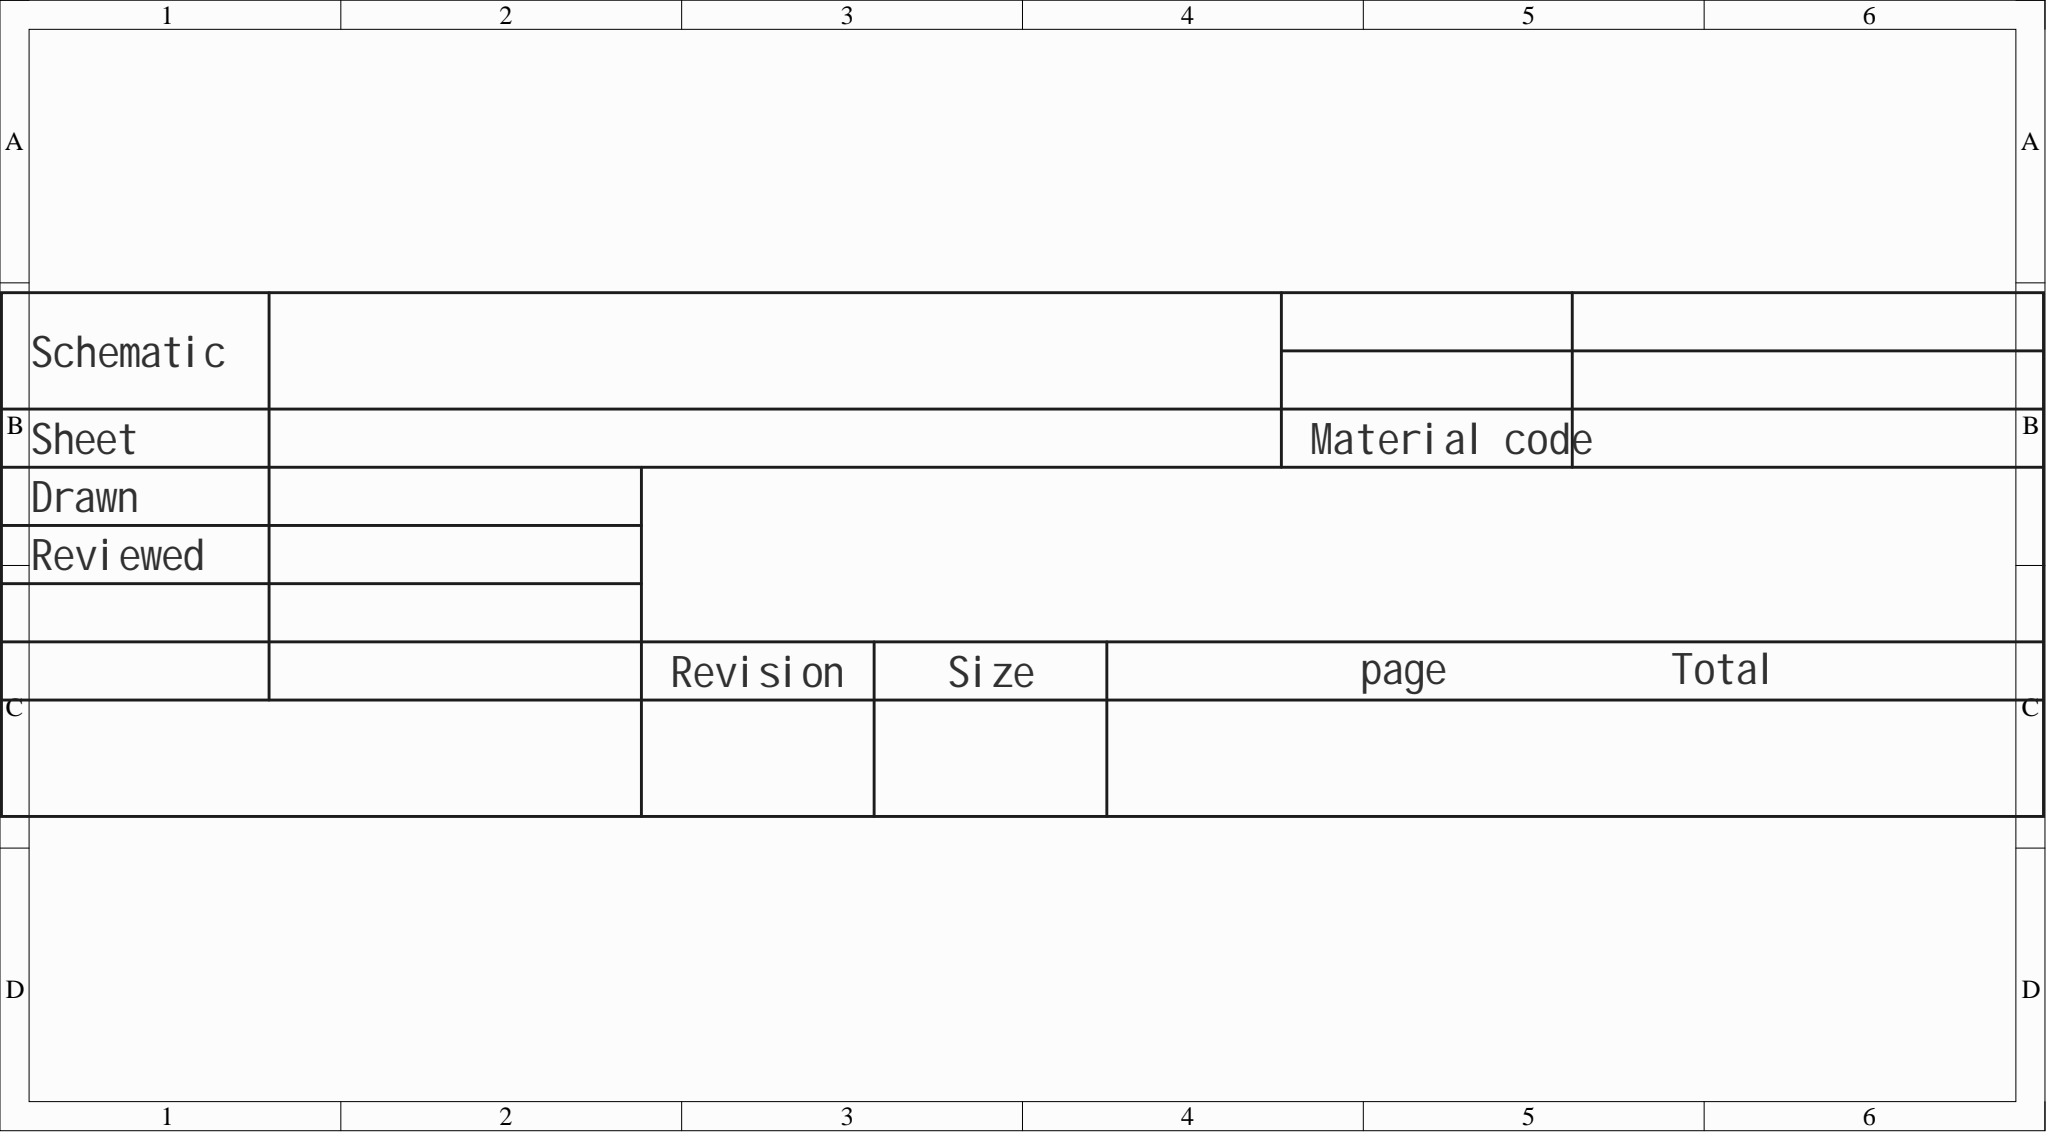Circuit board | Altium Designer | 22 parts | 24 nets
Bill of materials:
Comment,Description,Designator,Footprint,LibRef,Quantity
"buzzer-12X9","","BUZZER1","BUZ-TH_BD12.0-P7.60-D0.6-FD","buzzer-12X9","1"
"10uF","Capacitance: 10uF; Tolerance: ±20%; Rated voltage: 250V; Ripple current: -; Equivalent series resistance: -;","C4","CAP-TH_BD6.3-P2.50-D1.0-FD","LKMC1202E100MF","1"
"30pF","Capacitance: 30pF; Tolerance: ±5%; Rated voltage: 50V; Temperature coefficient: C0G;","C5, C6","CAP-TH_L3.6-W2.3-P5.00-D0.5","K300J10C0GF5UH5","2"
"22pF","","C7","C0603","CAP_0603","1"
"","","H1","HDR-TH_6P-P2.54-V-F","HDR-F_2.54_1x6P","1"
"LMB162ADC","16x2 character LCD module","LCD1","LCD1602","LMB162ADC","1"
"","","Q1","S8550P_SOT","S8550_SOT_PNP","1"
"1kΩ","","R30","Res_1/8W","Res_AXIAL-1/8W","1"
"10kΩ","","R39, R40","Res_1/8W","Res_AXIAL-1/8W","2"
"51K","","R41","R0603","Res_0603","1"
"-","Number of resistors: -; Resistance: -; Power per element: -;","RN1","RES-ARRAY-TH_9P-P2.54-D1.0","排阻 10 K 5%","1"
"Tact switch, 6*6*5 plastic head, 260G, travel 0.25mm, through-hole, middle 2 pins","","SW7, SW8, SW9, SW10, SW11","KEY-TH_2P-L6.0-W6.0-P5.00","轻触开关,6*6*5塑头,260G,行程0.25mm,直插中2脚","5"
"12MHz","Frequency: 12MHz; Frequency tolerance (room temp): ±30ppm; External load capacitance: -; Frequency stability (full temp): ±50ppm;","U2","HC-49US_L11.0-W4.6-P4.88","ECS-120-S-4","1"
"STC89C516RD+40I-PDIP40","CPU core: 51 series; Program memory capacity: 61KB; Total RAM: 1.25KB; GPIO port count: 35; Operating voltage range: 3.5V~5.5V; Max CPU clock: -; Program memory type: FLASH;","U3","DIP-40_L52.3-W13.9-P2.54-LS15.2-BL","STC89C516RD+40I-PDIP40","1"
"DS18B20","","U4","TO-92-3_L4.6-W3.6-P1.27-L-1","DS18B20","1"
"ADC0832BCN","","U5","PDIP-8_L9.6-W6.4-P2.54-LS7.6-BL","ADC0832BCN","1"
Netlist (Protel format):
[
BUZZER1
BUZ-TH_BD12.0-P7.60-D0.6-FD
buzzer-12X9



]
[
C4
CAP-TH_BD6.3-P2.50-D1.0-FD
10uF



]
[
C5
CAP-TH_L3.6-W2.3-P5.00-D0.5
30pF



]
[
C6
CAP-TH_L3.6-W2.3-P5.00-D0.5
30pF



]
[
C7
C0603
22pF



]
[
H1
HDR-TH_6P-P2.54-V-F




]
[
LCD1
LCD1602
LMB162ADC



]
[
Q1
S8550P_SOT




]
[
R30
Res_1/8W
1kΩ



]
[
R39
Res_1/8W
10kΩ



]
[
R40
Res_1/8W
10kΩ



]
[
R41
R0603
51K



]
[
RN1
RES-ARRAY-TH_9P-P2.54-D1.0
-



]
[
SW7
KEY-TH_2P-L6.0-W6.0-P5.00
Tact switch, 6*6*5 plastic head, 260G, travel 0.25mm, through-hole, middle 2 pins



]
[
SW8
KEY-TH_2P-L6.0-W6.0-P5.00
Tact switch, 6*6*5 plastic head, 260G, travel 0.25mm, through-hole, middle 2 pins



]
[
SW9
KEY-TH_2P-L6.0-W6.0-P5.00
Tact switch, 6*6*5 plastic head, 260G, travel 0.25mm, through-hole, middle 2 pins



]
[
SW10
KEY-TH_2P-L6.0-W6.0-P5.00
Tact switch, 6*6*5 plastic head, 260G, travel 0.25mm, through-hole, middle 2 pins



]
[
SW11
KEY-TH_2P-L6.0-W6.0-P5.00
Tact switch, 6*6*5 plastic head, 260G, travel 0.25mm, through-hole, middle 2 pins



]
[
U2
HC-49US_L11.0-W4.6-P4.88
12MHz



]
[
U3
DIP-40_L52.3-W13.9-P2.54-LS15.2-BL
STC89C516RD+40I-PDIP40



]
[
U4
TO-92-3_L4.6-W3.6-P1.27-L-1
DS18B20



]
[
U5
PDIP-8_L9.6-W6.4-P2.54-LS7.6-BL
ADC0832BCN



]
(
VCC
BUZZER1-1
C4-1
H1-3
LCD1-2
LCD1-15
R40-2
RN1-1
SW11-1
U3-40
U4-3
U5-8
)
(
NetU3_25
U3-25
U5-5
U5-6
)
(
NetU3_24
U3-24
U5-7
)
(
NetU3_23
U3-23
U5-1
)
(
NetU3_17
U3-17
U4-2
)
(
NetSW10_2
SW10-2
U3-10
)
(
NetSW9_2
SW9-2
U3-11
)
(
NetSW8_2
SW8-2
U3-12
)
(
NetSW7_2
SW7-2
U3-8
)
(
NetLCD1_14
LCD1-14
RN1-9
U3-32
)
(
NetLCD1_13
LCD1-13
RN1-8
U3-33
)
(
NetLCD1_12
LCD1-12
RN1-7
U3-34
)
(
NetLCD1_11
LCD1-11
RN1-6
U3-35
)
(
NetLCD1_10
LCD1-10
RN1-5
U3-36
)
(
NetLCD1_9
LCD1-9
RN1-4
U3-37
)
(
NetLCD1_8
LCD1-8
RN1-3
U3-38
)
(
NetLCD1_7
LCD1-7
RN1-2
U3-39
)
(
NetLCD1_3
LCD1-3
R30-2
R40-1
)
(
NetC7_2
C7-2
H1-1
R41-2
U5-2
)
(
NetC6_2
C6-2
U2-2
U3-19
)
(
NetC5_2
C5-2
U2-1
U3-18
)
(
NetC4_2
C4-2
R39-2
SW11-2
U3-9
)
(
NetBUZZER1_2
BUZZER1-2
Q1-2
)
(
GND
C5-1
C6-1
C7-1
H1-2
LCD1-1
LCD1-16
Q1-3
R30-1
R39-1
R41-1
SW7-1
SW8-1
SW9-1
SW10-1
U3-20
U4-1
U5-4
)